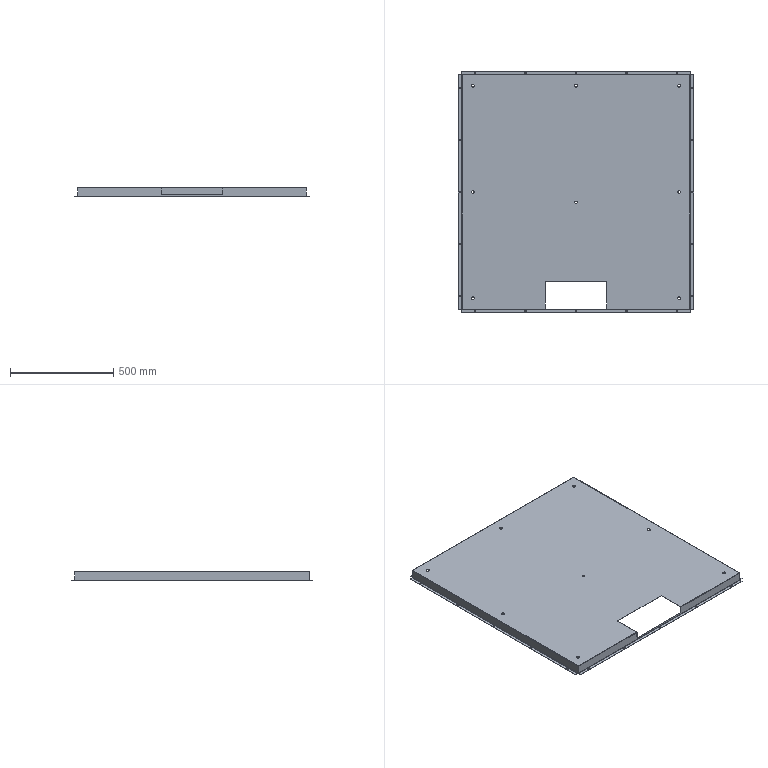Part | 1 solid | 186 faces | box 1140 x 1170 x 44 mm | volume 1469205 mm3 | plane 94 | cylinder 84 | spline 8 | commonest cylinder face diameters 7 x50 14 x14 1 x9 3 x9 11 x2